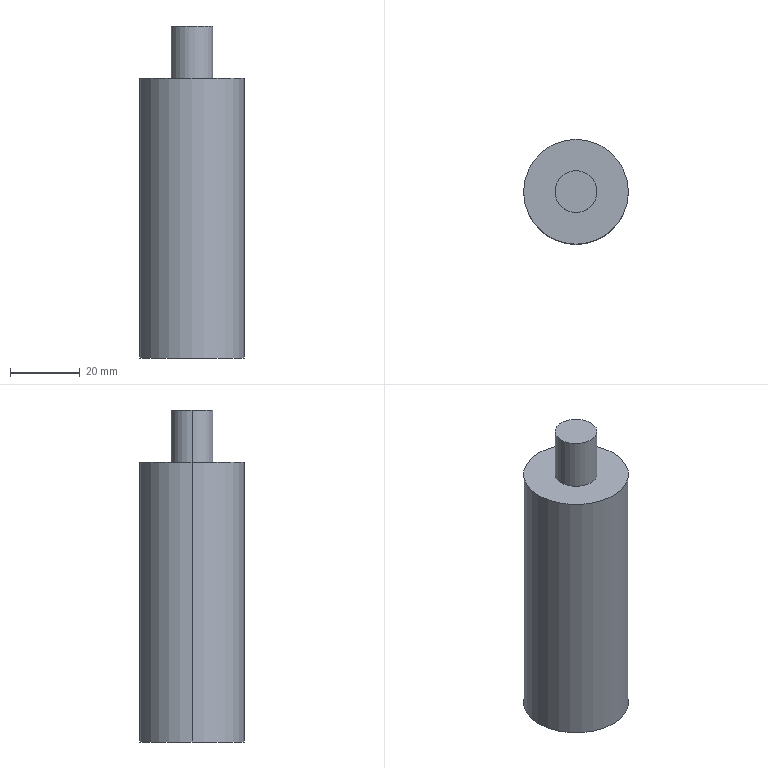Part | SolidWorks | features Extrusion 1, HoleWzd 1, ICE 1 | 1 solid | 11 faces | box 30 x 30 x 95 mm | volume 57062 mm3 | cylinder 6 | plane 3 | cone 2 | commonest cylinder face diameters 8.5 x2 12 x2 30 x2
STEP:
#1=CARTESIAN_POINT('',(6.,0.,55.));
#2=VERTEX_POINT('',#1);
#3=CARTESIAN_POINT('',(-6.,0.,55.));
#4=VERTEX_POINT('',#3);
#5=CARTESIAN_POINT('',(0.,0.,55.));
#6=DIRECTION('',(0.,0.,1.));
#7=DIRECTION('',(1.,0.,0.));
#8=AXIS2_PLACEMENT_3D('',#5,#6,#7);
#9=CIRCLE('',#8,6.);
#10=EDGE_CURVE('',#2,#4,#9,.T.);
#11=ORIENTED_EDGE('',*,*,#10,.F.);
#12=CARTESIAN_POINT('',(6.,0.,40.));
#13=VERTEX_POINT('',#12);
#14=CARTESIAN_POINT('',(6.,0.,55.));
#15=DIRECTION('',(0.,0.,-1.));
#16=VECTOR('',#15,1000.);
#17=LINE('',#14,#16);
#18=EDGE_CURVE('',#2,#13,#17,.T.);
#19=ORIENTED_EDGE('',*,*,#18,.T.);
#20=CARTESIAN_POINT('',(-6.,0.,40.));
#21=VERTEX_POINT('',#20);
#22=CARTESIAN_POINT('',(0.,0.,40.));
#23=DIRECTION('',(0.,0.,1.));
#24=DIRECTION('',(1.,0.,0.));
#25=AXIS2_PLACEMENT_3D('',#22,#23,#24);
#26=CIRCLE('',#25,6.);
#27=EDGE_CURVE('',#13,#21,#26,.T.);
#28=ORIENTED_EDGE('',*,*,#27,.T.);
#29=CARTESIAN_POINT('',(-6.,0.,55.));
#30=DIRECTION('',(0.,0.,-1.));
#31=VECTOR('',#30,1000.);
#32=LINE('',#29,#31);
#33=EDGE_CURVE('',#4,#21,#32,.T.);
#34=ORIENTED_EDGE('',*,*,#33,.F.);
#35=EDGE_LOOP('',(#11,#19,#28,#34));
#36=FACE_OUTER_BOUND('',#35,.T.);
#37=CARTESIAN_POINT('',(0.,0.,55.));
#38=DIRECTION('',(0.,0.,-1.));
#39=DIRECTION('',(-1.,0.,0.));
#40=AXIS2_PLACEMENT_3D('',#37,#38,#39);
#41=CYLINDRICAL_SURFACE('',#40,6.);
#42=ADVANCED_FACE('',(#36),#41,.T.);
#43=CARTESIAN_POINT('',(4.25,0.,-20.));
#44=VERTEX_POINT('',#43);
#45=CARTESIAN_POINT('',(-4.25,0.,-20.));
#46=VERTEX_POINT('',#45);
#47=CARTESIAN_POINT('',(0.,0.,-20.));
#48=DIRECTION('',(0.,0.,-1.));
#49=DIRECTION('',(-1.,0.,0.));
#50=AXIS2_PLACEMENT_3D('',#47,#48,#49);
#51=CIRCLE('',#50,4.25);
#52=EDGE_CURVE('',#44,#46,#51,.T.);
#53=ORIENTED_EDGE('',*,*,#52,.F.);
#54=CARTESIAN_POINT('',(4.25,0.,-40.));
#55=VERTEX_POINT('',#54);
#56=CARTESIAN_POINT('',(4.25,0.,-40.));
#57=DIRECTION('',(0.,0.,-1.));
#58=VECTOR('',#57,1000.);
#59=LINE('',#56,#58);
#60=EDGE_CURVE('',#44,#55,#59,.T.);
#61=ORIENTED_EDGE('',*,*,#60,.T.);
#62=CARTESIAN_POINT('',(-4.25,0.,-40.));
#63=VERTEX_POINT('',#62);
#64=CARTESIAN_POINT('',(0.,0.,-40.));
#65=DIRECTION('',(0.,0.,-1.));
#66=DIRECTION('',(-1.,0.,0.));
#67=AXIS2_PLACEMENT_3D('',#64,#65,#66);
#68=CIRCLE('',#67,4.25);
#69=EDGE_CURVE('',#55,#63,#68,.T.);
#70=ORIENTED_EDGE('',*,*,#69,.T.);
#71=CARTESIAN_POINT('',(-4.25,0.,-40.));
#72=DIRECTION('',(0.,0.,-1.));
#73=VECTOR('',#72,1000.);
#74=LINE('',#71,#73);
#75=EDGE_CURVE('',#46,#63,#74,.T.);
#76=ORIENTED_EDGE('',*,*,#75,.F.);
#77=EDGE_LOOP('',(#53,#61,#70,#76));
#78=FACE_OUTER_BOUND('',#77,.T.);
#79=CARTESIAN_POINT('',(0.,0.,-40.));
#80=DIRECTION('',(0.,0.,-1.));
#81=DIRECTION('',(-1.,0.,0.));
#82=AXIS2_PLACEMENT_3D('',#79,#80,#81);
#83=CYLINDRICAL_SURFACE('',#82,4.25);
#84=ADVANCED_FACE('',(#78),#83,.F.);
#85=CARTESIAN_POINT('',(0.,0.,-17.446));
#86=VERTEX_POINT('',#85);
#87=CARTESIAN_POINT('',(-4.25,0.,-20.));
#88=DIRECTION('',(-0.8572,0.,-0.515));
#89=VECTOR('',#88,1000.);
#90=LINE('',#87,#89);
#91=EDGE_CURVE('',#86,#46,#90,.T.);
#92=ORIENTED_EDGE('',*,*,#91,.F.);
#93=CARTESIAN_POINT('',(4.25,0.,-20.));
#94=DIRECTION('',(0.8572,0.,-0.515));
#95=VECTOR('',#94,1000.);
#96=LINE('',#93,#95);
#97=EDGE_CURVE('',#86,#44,#96,.T.);
#98=ORIENTED_EDGE('',*,*,#97,.T.);
#99=ORIENTED_EDGE('',*,*,#52,.T.);
#100=EDGE_LOOP('',(#92,#98,#99));
#101=FACE_OUTER_BOUND('',#100,.T.);
#102=CARTESIAN_POINT('',(0.,0.,-20.));
#103=DIRECTION('',(0.,0.,-1.));
#104=DIRECTION('',(-1.,0.,0.));
#105=AXIS2_PLACEMENT_3D('',#102,#103,#104);
#106=CONICAL_SURFACE('',#105,4.25,1.03);
#107=ADVANCED_FACE('',(#101),#106,.F.);
#108=CARTESIAN_POINT('',(15.,0.,40.));
#109=VERTEX_POINT('',#108);
#110=CARTESIAN_POINT('',(-15.,0.,40.));
#111=VERTEX_POINT('',#110);
#112=CARTESIAN_POINT('',(0.,0.,40.));
#113=DIRECTION('',(0.,0.,1.));
#114=DIRECTION('',(1.,0.,0.));
#115=AXIS2_PLACEMENT_3D('',#112,#113,#114);
#116=CIRCLE('',#115,15.);
#117=EDGE_CURVE('',#109,#111,#116,.T.);
#118=ORIENTED_EDGE('',*,*,#117,.F.);
#119=CARTESIAN_POINT('',(15.,0.,-40.));
#120=VERTEX_POINT('',#119);
#121=CARTESIAN_POINT('',(15.,0.,40.));
#122=DIRECTION('',(0.,0.,-1.));
#123=VECTOR('',#122,1000.);
#124=LINE('',#121,#123);
#125=EDGE_CURVE('',#109,#120,#124,.T.);
#126=ORIENTED_EDGE('',*,*,#125,.T.);
#127=CARTESIAN_POINT('',(-15.,0.,-40.));
#128=VERTEX_POINT('',#127);
#129=CARTESIAN_POINT('',(0.,0.,-40.));
#130=DIRECTION('',(0.,0.,1.));
#131=DIRECTION('',(1.,0.,0.));
#132=AXIS2_PLACEMENT_3D('',#129,#130,#131);
#133=CIRCLE('',#132,15.);
#134=EDGE_CURVE('',#120,#128,#133,.T.);
#135=ORIENTED_EDGE('',*,*,#134,.T.);
#136=CARTESIAN_POINT('',(-15.,0.,40.));
#137=DIRECTION('',(0.,0.,-1.));
#138=VECTOR('',#137,1000.);
#139=LINE('',#136,#138);
#140=EDGE_CURVE('',#111,#128,#139,.T.);
#141=ORIENTED_EDGE('',*,*,#140,.F.);
#142=EDGE_LOOP('',(#118,#126,#135,#141));
#143=FACE_OUTER_BOUND('',#142,.T.);
#144=CARTESIAN_POINT('',(0.,0.,40.));
#145=DIRECTION('',(0.,0.,-1.));
#146=DIRECTION('',(-1.,0.,0.));
#147=AXIS2_PLACEMENT_3D('',#144,#145,#146);
#148=CYLINDRICAL_SURFACE('',#147,15.);
#149=ADVANCED_FACE('',(#143),#148,.T.);
#150=ORIENTED_EDGE('',*,*,#125,.F.);
#151=CARTESIAN_POINT('',(0.,0.,40.));
#152=DIRECTION('',(0.,0.,1.));
#153=DIRECTION('',(1.,0.,0.));
#154=AXIS2_PLACEMENT_3D('',#151,#152,#153);
#155=CIRCLE('',#154,15.);
#156=EDGE_CURVE('',#111,#109,#155,.T.);
#157=ORIENTED_EDGE('',*,*,#156,.F.);
#158=ORIENTED_EDGE('',*,*,#140,.T.);
#159=CARTESIAN_POINT('',(0.,0.,-40.));
#160=DIRECTION('',(0.,0.,1.));
#161=DIRECTION('',(1.,0.,0.));
#162=AXIS2_PLACEMENT_3D('',#159,#160,#161);
#163=CIRCLE('',#162,15.);
#164=EDGE_CURVE('',#128,#120,#163,.T.);
#165=ORIENTED_EDGE('',*,*,#164,.T.);
#166=EDGE_LOOP('',(#150,#157,#158,#165));
#167=FACE_OUTER_BOUND('',#166,.T.);
#168=CARTESIAN_POINT('',(0.,0.,40.));
#169=DIRECTION('',(0.,0.,-1.));
#170=DIRECTION('',(-1.,0.,0.));
#171=AXIS2_PLACEMENT_3D('',#168,#169,#170);
#172=CYLINDRICAL_SURFACE('',#171,15.);
#173=ADVANCED_FACE('',(#167),#172,.T.);
#174=CARTESIAN_POINT('',(0.,0.,40.));
#175=DIRECTION('',(0.,0.,1.));
#176=DIRECTION('',(1.,0.,0.));
#177=AXIS2_PLACEMENT_3D('',#174,#175,#176);
#178=CIRCLE('',#177,6.);
#179=EDGE_CURVE('',#21,#13,#178,.T.);
#180=ORIENTED_EDGE('',*,*,#179,.F.);
#181=ORIENTED_EDGE('',*,*,#27,.F.);
#182=EDGE_LOOP('',(#180,#181));
#183=FACE_BOUND('',#182,.T.);
#184=ORIENTED_EDGE('',*,*,#156,.T.);
#185=ORIENTED_EDGE('',*,*,#117,.T.);
#186=EDGE_LOOP('',(#184,#185));
#187=FACE_OUTER_BOUND('',#186,.T.);
#188=CARTESIAN_POINT('',(0.,0.,40.));
#189=DIRECTION('',(0.,0.,1.));
#190=DIRECTION('',(1.,0.,0.));
#191=AXIS2_PLACEMENT_3D('',#188,#189,#190);
#192=PLANE('',#191);
#193=ADVANCED_FACE('',(#183,#187),#192,.T.);
#194=CARTESIAN_POINT('',(0.,0.,-40.));
#195=DIRECTION('',(0.,0.,-1.));
#196=DIRECTION('',(-1.,0.,0.));
#197=AXIS2_PLACEMENT_3D('',#194,#195,#196);
#198=CIRCLE('',#197,4.25);
#199=EDGE_CURVE('',#63,#55,#198,.T.);
#200=ORIENTED_EDGE('',*,*,#199,.F.);
#201=ORIENTED_EDGE('',*,*,#69,.F.);
#202=EDGE_LOOP('',(#200,#201));
#203=FACE_BOUND('',#202,.T.);
#204=ORIENTED_EDGE('',*,*,#164,.F.);
#205=ORIENTED_EDGE('',*,*,#134,.F.);
#206=EDGE_LOOP('',(#204,#205));
#207=FACE_OUTER_BOUND('',#206,.T.);
#208=CARTESIAN_POINT('',(0.,0.,-40.));
#209=DIRECTION('',(0.,0.,1.));
#210=DIRECTION('',(1.,0.,0.));
#211=AXIS2_PLACEMENT_3D('',#208,#209,#210);
#212=PLANE('',#211);
#213=ADVANCED_FACE('',(#203,#207),#212,.F.);
#214=ORIENTED_EDGE('',*,*,#97,.F.);
#215=ORIENTED_EDGE('',*,*,#91,.T.);
#216=CARTESIAN_POINT('',(0.,0.,-20.));
#217=DIRECTION('',(0.,0.,-1.));
#218=DIRECTION('',(-1.,0.,0.));
#219=AXIS2_PLACEMENT_3D('',#216,#217,#218);
#220=CIRCLE('',#219,4.25);
#221=EDGE_CURVE('',#46,#44,#220,.T.);
#222=ORIENTED_EDGE('',*,*,#221,.T.);
#223=EDGE_LOOP('',(#214,#215,#222));
#224=FACE_OUTER_BOUND('',#223,.T.);
#225=CARTESIAN_POINT('',(0.,0.,-20.));
#226=DIRECTION('',(0.,0.,-1.));
#227=DIRECTION('',(-1.,0.,0.));
#228=AXIS2_PLACEMENT_3D('',#225,#226,#227);
#229=CONICAL_SURFACE('',#228,4.25,1.03);
#230=ADVANCED_FACE('',(#224),#229,.F.);
#231=ORIENTED_EDGE('',*,*,#60,.F.);
#232=ORIENTED_EDGE('',*,*,#221,.F.);
#233=ORIENTED_EDGE('',*,*,#75,.T.);
#234=ORIENTED_EDGE('',*,*,#199,.T.);
#235=EDGE_LOOP('',(#231,#232,#233,#234));
#236=FACE_OUTER_BOUND('',#235,.T.);
#237=CARTESIAN_POINT('',(0.,0.,-40.));
#238=DIRECTION('',(0.,0.,-1.));
#239=DIRECTION('',(-1.,0.,0.));
#240=AXIS2_PLACEMENT_3D('',#237,#238,#239);
#241=CYLINDRICAL_SURFACE('',#240,4.25);
#242=ADVANCED_FACE('',(#236),#241,.F.);
#243=ORIENTED_EDGE('',*,*,#18,.F.);
#244=CARTESIAN_POINT('',(0.,0.,55.));
#245=DIRECTION('',(0.,0.,1.));
#246=DIRECTION('',(1.,0.,0.));
#247=AXIS2_PLACEMENT_3D('',#244,#245,#246);
#248=CIRCLE('',#247,6.);
#249=EDGE_CURVE('',#4,#2,#248,.T.);
#250=ORIENTED_EDGE('',*,*,#249,.F.);
#251=ORIENTED_EDGE('',*,*,#33,.T.);
#252=ORIENTED_EDGE('',*,*,#179,.T.);
#253=EDGE_LOOP('',(#243,#250,#251,#252));
#254=FACE_OUTER_BOUND('',#253,.T.);
#255=CARTESIAN_POINT('',(0.,0.,55.));
#256=DIRECTION('',(0.,0.,-1.));
#257=DIRECTION('',(-1.,0.,0.));
#258=AXIS2_PLACEMENT_3D('',#255,#256,#257);
#259=CYLINDRICAL_SURFACE('',#258,6.);
#260=ADVANCED_FACE('',(#254),#259,.T.);
#261=ORIENTED_EDGE('',*,*,#249,.T.);
#262=ORIENTED_EDGE('',*,*,#10,.T.);
#263=EDGE_LOOP('',(#261,#262));
#264=FACE_OUTER_BOUND('',#263,.T.);
#265=CARTESIAN_POINT('',(0.,0.,55.));
#266=DIRECTION('',(0.,0.,1.));
#267=DIRECTION('',(1.,0.,0.));
#268=AXIS2_PLACEMENT_3D('',#265,#266,#267);
#269=PLANE('',#268);
#270=ADVANCED_FACE('',(#264),#269,.T.);
#271=CLOSED_SHELL('',(#42,#84,#107,#149,#173,#193,#213,#230,#242,#260,#270));
#272=MANIFOLD_SOLID_BREP('',#271);
#273=CARTESIAN_POINT('',(0.,0.,0.));
#274=DIRECTION('',(0.,0.,1.));
#275=DIRECTION('',(1.,0.,0.));
#276=AXIS2_PLACEMENT_3D('',#273,#274,#275);
#277=(LENGTH_UNIT()NAMED_UNIT(*)SI_UNIT(.MILLI.,.METRE.));
#278=UNCERTAINTY_MEASURE_WITH_UNIT(LENGTH_MEASURE(0.00001),#277,'','');
#279=(NAMED_UNIT(*)PLANE_ANGLE_UNIT()SI_UNIT($,.RADIAN.));
#280=(NAMED_UNIT(*)SI_UNIT($,.STERADIAN.)SOLID_ANGLE_UNIT());
#281=(GEOMETRIC_REPRESENTATION_CONTEXT(3)GLOBAL_UNCERTAINTY_ASSIGNED_CONTEXT((#278))GLOBAL_UNIT_ASSIGNED_CONTEXT((#277,#279,#280))REPRESENTATION_CONTEXT('',''));
#282=ADVANCED_BREP_SHAPE_REPRESENTATION('',(#272,#276),#281);